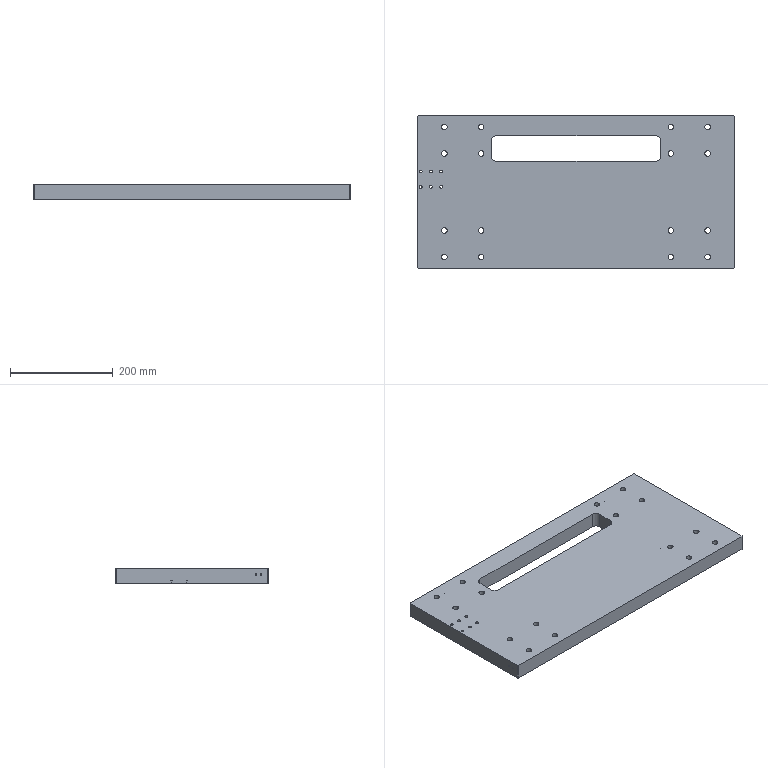Part | SolidWorks | features HoleWzd 9, Chamfer 1, Extrusion 1, ICE 1, LPattern 1, MirrorPattern 1 | 1 solid | 320 faces | box 620 x 300 x 30 mm | volume 4982142 mm3 | cylinder 188 | cone 96 | plane 36 | commonest cylinder face diameters 4.2 x60 11 x32 18 x32 10.2 x16 5.5 x12 10 x12